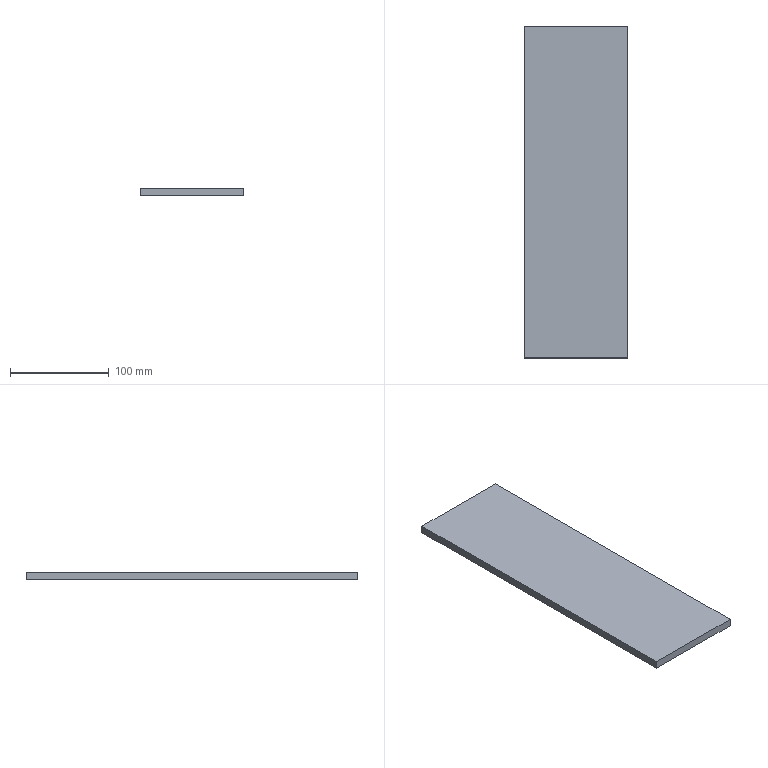Part | SolidWorks | features Extrusion 1 | 1 solid | 6 faces | box 105 x 336 x 8 mm | volume 282240 mm3 | plane 6
STEP:
#1=CARTESIAN_POINT('',(-52.5,168.,-4.));
#2=VERTEX_POINT('',#1);
#3=CARTESIAN_POINT('',(-52.5,-168.,-4.));
#4=VERTEX_POINT('',#3);
#5=CARTESIAN_POINT('',(-52.5,168.,-4.));
#6=DIRECTION('',(0.,-1.,0.));
#7=VECTOR('',#6,1000.);
#8=LINE('',#5,#7);
#9=EDGE_CURVE('',#2,#4,#8,.T.);
#10=ORIENTED_EDGE('',*,*,#9,.T.);
#11=CARTESIAN_POINT('',(-52.5,-168.,4.));
#12=VERTEX_POINT('',#11);
#13=CARTESIAN_POINT('',(-52.5,-168.,4.));
#14=DIRECTION('',(0.,0.,-1.));
#15=VECTOR('',#14,1000.);
#16=LINE('',#13,#15);
#17=EDGE_CURVE('',#12,#4,#16,.T.);
#18=ORIENTED_EDGE('',*,*,#17,.F.);
#19=CARTESIAN_POINT('',(-52.5,168.,4.));
#20=VERTEX_POINT('',#19);
#21=CARTESIAN_POINT('',(-52.5,168.,4.));
#22=DIRECTION('',(0.,-1.,0.));
#23=VECTOR('',#22,1000.);
#24=LINE('',#21,#23);
#25=EDGE_CURVE('',#20,#12,#24,.T.);
#26=ORIENTED_EDGE('',*,*,#25,.F.);
#27=CARTESIAN_POINT('',(-52.5,168.,4.));
#28=DIRECTION('',(0.,0.,-1.));
#29=VECTOR('',#28,1000.);
#30=LINE('',#27,#29);
#31=EDGE_CURVE('',#20,#2,#30,.T.);
#32=ORIENTED_EDGE('',*,*,#31,.T.);
#33=EDGE_LOOP('',(#10,#18,#26,#32));
#34=FACE_OUTER_BOUND('',#33,.T.);
#35=CARTESIAN_POINT('',(-52.5,168.,4.));
#36=DIRECTION('',(1.,0.,0.));
#37=DIRECTION('',(0.,1.,0.));
#38=AXIS2_PLACEMENT_3D('',#35,#36,#37);
#39=PLANE('',#38);
#40=ADVANCED_FACE('',(#34),#39,.F.);
#41=CARTESIAN_POINT('',(52.5,-168.,-4.));
#42=VERTEX_POINT('',#41);
#43=CARTESIAN_POINT('',(-52.5,-168.,-4.));
#44=DIRECTION('',(1.,0.,0.));
#45=VECTOR('',#44,1000.);
#46=LINE('',#43,#45);
#47=EDGE_CURVE('',#4,#42,#46,.T.);
#48=ORIENTED_EDGE('',*,*,#47,.T.);
#49=CARTESIAN_POINT('',(52.5,-168.,4.));
#50=VERTEX_POINT('',#49);
#51=CARTESIAN_POINT('',(52.5,-168.,4.));
#52=DIRECTION('',(0.,0.,-1.));
#53=VECTOR('',#52,1000.);
#54=LINE('',#51,#53);
#55=EDGE_CURVE('',#50,#42,#54,.T.);
#56=ORIENTED_EDGE('',*,*,#55,.F.);
#57=CARTESIAN_POINT('',(-52.5,-168.,4.));
#58=DIRECTION('',(1.,0.,0.));
#59=VECTOR('',#58,1000.);
#60=LINE('',#57,#59);
#61=EDGE_CURVE('',#12,#50,#60,.T.);
#62=ORIENTED_EDGE('',*,*,#61,.F.);
#63=ORIENTED_EDGE('',*,*,#17,.T.);
#64=EDGE_LOOP('',(#48,#56,#62,#63));
#65=FACE_OUTER_BOUND('',#64,.T.);
#66=CARTESIAN_POINT('',(-52.5,-168.,4.));
#67=DIRECTION('',(0.,1.,0.));
#68=DIRECTION('',(-1.,0.,0.));
#69=AXIS2_PLACEMENT_3D('',#66,#67,#68);
#70=PLANE('',#69);
#71=ADVANCED_FACE('',(#65),#70,.F.);
#72=CARTESIAN_POINT('',(52.5,168.,-4.));
#73=VERTEX_POINT('',#72);
#74=CARTESIAN_POINT('',(52.5,168.,-4.));
#75=DIRECTION('',(0.,1.,0.));
#76=VECTOR('',#75,1000.);
#77=LINE('',#74,#76);
#78=EDGE_CURVE('',#42,#73,#77,.T.);
#79=ORIENTED_EDGE('',*,*,#78,.T.);
#80=CARTESIAN_POINT('',(52.5,168.,4.));
#81=VERTEX_POINT('',#80);
#82=CARTESIAN_POINT('',(52.5,168.,4.));
#83=DIRECTION('',(0.,0.,-1.));
#84=VECTOR('',#83,1000.);
#85=LINE('',#82,#84);
#86=EDGE_CURVE('',#81,#73,#85,.T.);
#87=ORIENTED_EDGE('',*,*,#86,.F.);
#88=CARTESIAN_POINT('',(52.5,168.,4.));
#89=DIRECTION('',(0.,1.,0.));
#90=VECTOR('',#89,1000.);
#91=LINE('',#88,#90);
#92=EDGE_CURVE('',#50,#81,#91,.T.);
#93=ORIENTED_EDGE('',*,*,#92,.F.);
#94=ORIENTED_EDGE('',*,*,#55,.T.);
#95=EDGE_LOOP('',(#79,#87,#93,#94));
#96=FACE_OUTER_BOUND('',#95,.T.);
#97=CARTESIAN_POINT('',(52.5,168.,4.));
#98=DIRECTION('',(-1.,0.,0.));
#99=DIRECTION('',(0.,-1.,0.));
#100=AXIS2_PLACEMENT_3D('',#97,#98,#99);
#101=PLANE('',#100);
#102=ADVANCED_FACE('',(#96),#101,.F.);
#103=CARTESIAN_POINT('',(-52.5,168.,-4.));
#104=DIRECTION('',(-1.,0.,0.));
#105=VECTOR('',#104,1000.);
#106=LINE('',#103,#105);
#107=EDGE_CURVE('',#73,#2,#106,.T.);
#108=ORIENTED_EDGE('',*,*,#107,.T.);
#109=ORIENTED_EDGE('',*,*,#31,.F.);
#110=CARTESIAN_POINT('',(-52.5,168.,4.));
#111=DIRECTION('',(-1.,0.,0.));
#112=VECTOR('',#111,1000.);
#113=LINE('',#110,#112);
#114=EDGE_CURVE('',#81,#20,#113,.T.);
#115=ORIENTED_EDGE('',*,*,#114,.F.);
#116=ORIENTED_EDGE('',*,*,#86,.T.);
#117=EDGE_LOOP('',(#108,#109,#115,#116));
#118=FACE_OUTER_BOUND('',#117,.T.);
#119=CARTESIAN_POINT('',(-52.5,168.,4.));
#120=DIRECTION('',(0.,-1.,0.));
#121=DIRECTION('',(0.,0.,-1.));
#122=AXIS2_PLACEMENT_3D('',#119,#120,#121);
#123=PLANE('',#122);
#124=ADVANCED_FACE('',(#118),#123,.F.);
#125=ORIENTED_EDGE('',*,*,#25,.T.);
#126=ORIENTED_EDGE('',*,*,#61,.T.);
#127=ORIENTED_EDGE('',*,*,#92,.T.);
#128=ORIENTED_EDGE('',*,*,#114,.T.);
#129=EDGE_LOOP('',(#125,#126,#127,#128));
#130=FACE_OUTER_BOUND('',#129,.T.);
#131=CARTESIAN_POINT('',(-52.5,-168.,4.));
#132=DIRECTION('',(0.,0.,1.));
#133=DIRECTION('',(1.,0.,0.));
#134=AXIS2_PLACEMENT_3D('',#131,#132,#133);
#135=PLANE('',#134);
#136=ADVANCED_FACE('',(#130),#135,.T.);
#137=ORIENTED_EDGE('',*,*,#9,.F.);
#138=ORIENTED_EDGE('',*,*,#107,.F.);
#139=ORIENTED_EDGE('',*,*,#78,.F.);
#140=ORIENTED_EDGE('',*,*,#47,.F.);
#141=EDGE_LOOP('',(#137,#138,#139,#140));
#142=FACE_OUTER_BOUND('',#141,.T.);
#143=CARTESIAN_POINT('',(-52.5,-168.,-4.));
#144=DIRECTION('',(0.,0.,1.));
#145=DIRECTION('',(1.,0.,0.));
#146=AXIS2_PLACEMENT_3D('',#143,#144,#145);
#147=PLANE('',#146);
#148=ADVANCED_FACE('',(#142),#147,.F.);
#149=CLOSED_SHELL('',(#40,#71,#102,#124,#136,#148));
#150=MANIFOLD_SOLID_BREP('',#149);
#151=CARTESIAN_POINT('',(0.,0.,0.));
#152=DIRECTION('',(0.,0.,1.));
#153=DIRECTION('',(1.,0.,0.));
#154=AXIS2_PLACEMENT_3D('',#151,#152,#153);
#155=(LENGTH_UNIT()NAMED_UNIT(*)SI_UNIT(.MILLI.,.METRE.));
#156=UNCERTAINTY_MEASURE_WITH_UNIT(LENGTH_MEASURE(0.00001),#155,'','');
#157=(NAMED_UNIT(*)PLANE_ANGLE_UNIT()SI_UNIT($,.RADIAN.));
#158=(NAMED_UNIT(*)SI_UNIT($,.STERADIAN.)SOLID_ANGLE_UNIT());
#159=(GEOMETRIC_REPRESENTATION_CONTEXT(3)GLOBAL_UNCERTAINTY_ASSIGNED_CONTEXT((#156))GLOBAL_UNIT_ASSIGNED_CONTEXT((#155,#157,#158))REPRESENTATION_CONTEXT('',''));
#160=ADVANCED_BREP_SHAPE_REPRESENTATION('',(#150,#154),#159);